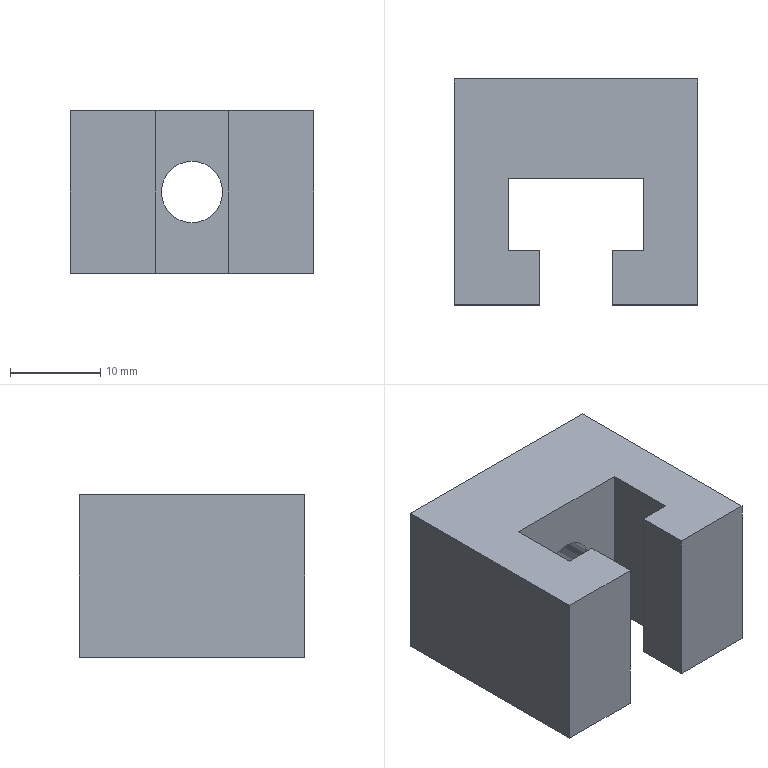Part | STEP file | iron shell displacement union seat | 1 solid | 16 faces | box 27 x 25 x 18 mm | volume 8727 mm3 | plane 14 | cylinder 2 | commonest cylinder face diameters 6.8 x2
STEP:
#1=CARTESIAN_POINT('',(0.,0.,0.));
#2=DIRECTION('',(0.,0.,1.));
#3=DIRECTION('',(1.,0.,0.));
#4=AXIS2_PLACEMENT_3D('',#1,#2,#3);
#5=CARTESIAN_POINT('',(-1856.966,-5970.89,12.4));
#6=VERTEX_POINT('',#5);
#7=CARTESIAN_POINT('',(-1856.966,-5959.89,12.4));
#8=VERTEX_POINT('',#7);
#9=CARTESIAN_POINT('',(-1856.966,-5959.89,12.4));
#10=DIRECTION('',(0.,1.,0.));
#11=VECTOR('',#10,1.);
#12=LINE('',#9,#11);
#13=CARTESIAN_POINT('',(-1856.966,-5959.89,9.));
#14=DIRECTION('',(0.,1.,0.));
#15=DIRECTION('',(0.,0.,1.));
#16=AXIS2_PLACEMENT_3D('',#13,#14,#15);
#17=CYLINDRICAL_SURFACE('',#16,3.4);
#18=CARTESIAN_POINT('',(6.283,0.));
#19=DIRECTION('',(0.,1.));
#20=VECTOR('',#19,1.);
#21=LINE('',#18,#20);
#22=(GEOMETRIC_REPRESENTATION_CONTEXT(2)PARAMETRIC_REPRESENTATION_CONTEXT()REPRESENTATION_CONTEXT('',''));
#23=DEFINITIONAL_REPRESENTATION('',(#21),#22);
#24=PCURVE('',#17,#23);
#25=CARTESIAN_POINT('',(-1856.966,-5959.89,9.));
#26=DIRECTION('',(0.,1.,0.));
#27=DIRECTION('',(0.,0.,1.));
#28=AXIS2_PLACEMENT_3D('',#25,#26,#27);
#29=CYLINDRICAL_SURFACE('',#28,3.4);
#30=CARTESIAN_POINT('',(0.,0.));
#31=DIRECTION('',(0.,1.));
#32=VECTOR('',#31,1.);
#33=LINE('',#30,#32);
#34=(GEOMETRIC_REPRESENTATION_CONTEXT(2)PARAMETRIC_REPRESENTATION_CONTEXT()REPRESENTATION_CONTEXT('',''));
#35=DEFINITIONAL_REPRESENTATION('',(#33),#34);
#36=PCURVE('',#29,#35);
#37=SURFACE_CURVE('',#12,(#24,#36),.PCURVE_S1.);
#38=EDGE_CURVE('',#6,#8,#37,.T.);
#39=ORIENTED_EDGE('',*,*,#38,.T.);
#40=CARTESIAN_POINT('',(-1856.966,-5959.89,5.6));
#41=VERTEX_POINT('',#40);
#42=CARTESIAN_POINT('',(-1856.966,-5959.89,9.));
#43=DIRECTION('',(0.,1.,0.));
#44=DIRECTION('',(0.,0.,1.));
#45=AXIS2_PLACEMENT_3D('',#42,#43,#44);
#46=CIRCLE('',#45,3.4);
#47=CARTESIAN_POINT('',(0.,0.));
#48=DIRECTION('',(1.,0.));
#49=VECTOR('',#48,1.);
#50=LINE('',#47,#49);
#51=(GEOMETRIC_REPRESENTATION_CONTEXT(2)PARAMETRIC_REPRESENTATION_CONTEXT()REPRESENTATION_CONTEXT('',''));
#52=DEFINITIONAL_REPRESENTATION('',(#50),#51);
#53=PCURVE('',#17,#52);
#54=CARTESIAN_POINT('',(-1870.466,-5959.89,18.));
#55=DIRECTION('',(0.,-1.,0.));
#56=DIRECTION('',(0.,0.,-1.));
#57=AXIS2_PLACEMENT_3D('',#54,#55,#56);
#58=PLANE('',#57);
#59=CARTESIAN_POINT('',(5.6,13.5));
#60=CARTESIAN_POINT('',(5.6,19.389));
#61=CARTESIAN_POINT('',(10.7,16.444));
#62=CARTESIAN_POINT('',(15.8,13.5));
#63=CARTESIAN_POINT('',(10.7,10.556));
#64=CARTESIAN_POINT('',(5.6,7.611));
#65=CARTESIAN_POINT('',(5.6,13.5));
#66=(BOUNDED_CURVE()B_SPLINE_CURVE(2,(#59,#60,#61,#62,#63,#64,#65),.UNSPECIFIED.,.T.,.F.)B_SPLINE_CURVE_WITH_KNOTS((1,2,2,2,2,1),(-2.094,0.,2.094,4.189,6.283,8.378),.UNSPECIFIED.)CURVE()GEOMETRIC_REPRESENTATION_ITEM()RATIONAL_B_SPLINE_CURVE((1.,0.5,1.,0.5,1.,0.5,1.))REPRESENTATION_ITEM(''));
#67=(GEOMETRIC_REPRESENTATION_CONTEXT(2)PARAMETRIC_REPRESENTATION_CONTEXT()REPRESENTATION_CONTEXT('',''));
#68=DEFINITIONAL_REPRESENTATION('',(#66),#67);
#69=PCURVE('',#58,#68);
#70=SURFACE_CURVE('',#46,(#53,#69),.PCURVE_S1.);
#71=EDGE_CURVE('',#41,#8,#70,.T.);
#72=ORIENTED_EDGE('',*,*,#71,.F.);
#73=CARTESIAN_POINT('',(-1856.966,-5970.89,5.6));
#74=VERTEX_POINT('',#73);
#75=CARTESIAN_POINT('',(-1856.966,-5959.89,5.6));
#76=DIRECTION('',(0.,1.,0.));
#77=VECTOR('',#76,1.);
#78=LINE('',#75,#77);
#79=CARTESIAN_POINT('',(3.142,0.));
#80=DIRECTION('',(0.,1.));
#81=VECTOR('',#80,1.);
#82=LINE('',#79,#81);
#83=(GEOMETRIC_REPRESENTATION_CONTEXT(2)PARAMETRIC_REPRESENTATION_CONTEXT()REPRESENTATION_CONTEXT('',''));
#84=DEFINITIONAL_REPRESENTATION('',(#82),#83);
#85=PCURVE('',#17,#84);
#86=CARTESIAN_POINT('',(3.142,0.));
#87=DIRECTION('',(0.,1.));
#88=VECTOR('',#87,1.);
#89=LINE('',#86,#88);
#90=(GEOMETRIC_REPRESENTATION_CONTEXT(2)PARAMETRIC_REPRESENTATION_CONTEXT()REPRESENTATION_CONTEXT('',''));
#91=DEFINITIONAL_REPRESENTATION('',(#89),#90);
#92=PCURVE('',#29,#91);
#93=SURFACE_CURVE('',#78,(#85,#92),.PCURVE_S1.);
#94=EDGE_CURVE('',#74,#41,#93,.T.);
#95=ORIENTED_EDGE('',*,*,#94,.F.);
#96=CARTESIAN_POINT('',(-1856.966,-5970.89,9.));
#97=DIRECTION('',(0.,1.,0.));
#98=DIRECTION('',(0.,0.,1.));
#99=AXIS2_PLACEMENT_3D('',#96,#97,#98);
#100=CIRCLE('',#99,3.4);
#101=CARTESIAN_POINT('',(0.,-11.));
#102=DIRECTION('',(1.,0.));
#103=VECTOR('',#102,1.);
#104=LINE('',#101,#103);
#105=(GEOMETRIC_REPRESENTATION_CONTEXT(2)PARAMETRIC_REPRESENTATION_CONTEXT()REPRESENTATION_CONTEXT('',''));
#106=DEFINITIONAL_REPRESENTATION('',(#104),#105);
#107=PCURVE('',#17,#106);
#108=CARTESIAN_POINT('',(-1849.466,-5970.89,18.));
#109=DIRECTION('',(0.,1.,0.));
#110=DIRECTION('',(0.,0.,1.));
#111=AXIS2_PLACEMENT_3D('',#108,#109,#110);
#112=PLANE('',#111);
#113=CARTESIAN_POINT('',(-9.,-7.5));
#114=DIRECTION('',(1.,0.));
#115=AXIS2_PLACEMENT_2D('',#113,#114);
#116=CIRCLE('',#115,3.4);
#117=(GEOMETRIC_REPRESENTATION_CONTEXT(2)PARAMETRIC_REPRESENTATION_CONTEXT()REPRESENTATION_CONTEXT('',''));
#118=DEFINITIONAL_REPRESENTATION('',(#116),#117);
#119=PCURVE('',#112,#118);
#120=SURFACE_CURVE('',#100,(#107,#119),.PCURVE_S1.);
#121=EDGE_CURVE('',#74,#6,#120,.T.);
#122=ORIENTED_EDGE('',*,*,#121,.T.);
#123=EDGE_LOOP('',(#39,#72,#95,#122));
#124=FACE_BOUND('',#123,.F.);
#125=ADVANCED_FACE('',(#124),#17,.F.);
#126=CARTESIAN_POINT('',(-1856.966,-5959.89,9.));
#127=DIRECTION('',(0.,1.,0.));
#128=DIRECTION('',(0.,0.,1.));
#129=AXIS2_PLACEMENT_3D('',#126,#127,#128);
#130=CIRCLE('',#129,3.4);
#131=CARTESIAN_POINT('',(5.6,13.5));
#132=CARTESIAN_POINT('',(5.6,19.389));
#133=CARTESIAN_POINT('',(10.7,16.444));
#134=CARTESIAN_POINT('',(15.8,13.5));
#135=CARTESIAN_POINT('',(10.7,10.556));
#136=CARTESIAN_POINT('',(5.6,7.611));
#137=CARTESIAN_POINT('',(5.6,13.5));
#138=(BOUNDED_CURVE()B_SPLINE_CURVE(2,(#131,#132,#133,#134,#135,#136,#137),.UNSPECIFIED.,.T.,.F.)B_SPLINE_CURVE_WITH_KNOTS((1,2,2,2,2,1),(-2.094,0.,2.094,4.189,6.283,8.378),.UNSPECIFIED.)CURVE()GEOMETRIC_REPRESENTATION_ITEM()RATIONAL_B_SPLINE_CURVE((1.,0.5,1.,0.5,1.,0.5,1.))REPRESENTATION_ITEM(''));
#139=(GEOMETRIC_REPRESENTATION_CONTEXT(2)PARAMETRIC_REPRESENTATION_CONTEXT()REPRESENTATION_CONTEXT('',''));
#140=DEFINITIONAL_REPRESENTATION('',(#138),#139);
#141=PCURVE('',#58,#140);
#142=CARTESIAN_POINT('',(0.,0.));
#143=DIRECTION('',(1.,0.));
#144=VECTOR('',#143,1.);
#145=LINE('',#142,#144);
#146=(GEOMETRIC_REPRESENTATION_CONTEXT(2)PARAMETRIC_REPRESENTATION_CONTEXT()REPRESENTATION_CONTEXT('',''));
#147=DEFINITIONAL_REPRESENTATION('',(#145),#146);
#148=PCURVE('',#29,#147);
#149=SURFACE_CURVE('',#130,(#141,#148),.PCURVE_S1.);
#150=EDGE_CURVE('',#8,#41,#149,.T.);
#151=ORIENTED_EDGE('',*,*,#150,.F.);
#152=ORIENTED_EDGE('',*,*,#71,.F.);
#153=EDGE_LOOP('',(#151,#152));
#154=FACE_BOUND('',#153,.T.);
#155=CARTESIAN_POINT('',(-1843.466,-5959.89,0.));
#156=VERTEX_POINT('',#155);
#157=CARTESIAN_POINT('',(-1870.466,-5959.89,0.));
#158=VERTEX_POINT('',#157);
#159=CARTESIAN_POINT('',(-1870.466,-5959.89,0.));
#160=DIRECTION('',(-1.,0.,0.));
#161=VECTOR('',#160,1.);
#162=LINE('',#159,#161);
#163=CARTESIAN_POINT('',(18.,0.));
#164=DIRECTION('',(0.,-1.));
#165=VECTOR('',#164,1.);
#166=LINE('',#163,#165);
#167=(GEOMETRIC_REPRESENTATION_CONTEXT(2)PARAMETRIC_REPRESENTATION_CONTEXT()REPRESENTATION_CONTEXT('',''));
#168=DEFINITIONAL_REPRESENTATION('',(#166),#167);
#169=PCURVE('',#58,#168);
#170=CARTESIAN_POINT('',(-1843.466,-5959.89,0.));
#171=DIRECTION('',(0.,0.,-1.));
#172=DIRECTION('',(-1.,0.,0.));
#173=AXIS2_PLACEMENT_3D('',#170,#171,#172);
#174=PLANE('',#173);
#175=CARTESIAN_POINT('',(27.,0.));
#176=DIRECTION('',(1.,0.));
#177=VECTOR('',#176,1.);
#178=LINE('',#175,#177);
#179=(GEOMETRIC_REPRESENTATION_CONTEXT(2)PARAMETRIC_REPRESENTATION_CONTEXT()REPRESENTATION_CONTEXT('',''));
#180=DEFINITIONAL_REPRESENTATION('',(#178),#179);
#181=PCURVE('',#174,#180);
#182=SURFACE_CURVE('',#162,(#169,#181),.PCURVE_S1.);
#183=EDGE_CURVE('',#156,#158,#182,.T.);
#184=ORIENTED_EDGE('',*,*,#183,.T.);
#185=CARTESIAN_POINT('',(-1870.466,-5959.89,18.));
#186=VERTEX_POINT('',#185);
#187=CARTESIAN_POINT('',(-1870.466,-5959.89,18.));
#188=DIRECTION('',(0.,0.,-1.));
#189=VECTOR('',#188,1.);
#190=LINE('',#187,#189);
#191=CARTESIAN_POINT('',(0.,0.));
#192=DIRECTION('',(1.,0.));
#193=VECTOR('',#192,1.);
#194=LINE('',#191,#193);
#195=(GEOMETRIC_REPRESENTATION_CONTEXT(2)PARAMETRIC_REPRESENTATION_CONTEXT()REPRESENTATION_CONTEXT('',''));
#196=DEFINITIONAL_REPRESENTATION('',(#194),#195);
#197=PCURVE('',#58,#196);
#198=CARTESIAN_POINT('',(-1870.466,-5959.89,18.));
#199=DIRECTION('',(1.,0.,0.));
#200=DIRECTION('',(0.,0.,-1.));
#201=AXIS2_PLACEMENT_3D('',#198,#199,#200);
#202=PLANE('',#201);
#203=CARTESIAN_POINT('',(0.,0.));
#204=DIRECTION('',(1.,0.));
#205=VECTOR('',#204,1.);
#206=LINE('',#203,#205);
#207=(GEOMETRIC_REPRESENTATION_CONTEXT(2)PARAMETRIC_REPRESENTATION_CONTEXT()REPRESENTATION_CONTEXT('',''));
#208=DEFINITIONAL_REPRESENTATION('',(#206),#207);
#209=PCURVE('',#202,#208);
#210=SURFACE_CURVE('',#190,(#197,#209),.PCURVE_S1.);
#211=EDGE_CURVE('',#186,#158,#210,.T.);
#212=ORIENTED_EDGE('',*,*,#211,.F.);
#213=CARTESIAN_POINT('',(-1843.466,-5959.89,18.));
#214=VERTEX_POINT('',#213);
#215=CARTESIAN_POINT('',(-1870.466,-5959.89,18.));
#216=DIRECTION('',(-1.,0.,0.));
#217=VECTOR('',#216,1.);
#218=LINE('',#215,#217);
#219=CARTESIAN_POINT('',(0.,0.));
#220=DIRECTION('',(0.,-1.));
#221=VECTOR('',#220,1.);
#222=LINE('',#219,#221);
#223=(GEOMETRIC_REPRESENTATION_CONTEXT(2)PARAMETRIC_REPRESENTATION_CONTEXT()REPRESENTATION_CONTEXT('',''));
#224=DEFINITIONAL_REPRESENTATION('',(#222),#223);
#225=PCURVE('',#58,#224);
#226=CARTESIAN_POINT('',(-1843.466,-5959.89,18.));
#227=DIRECTION('',(0.,0.,-1.));
#228=DIRECTION('',(-1.,0.,0.));
#229=AXIS2_PLACEMENT_3D('',#226,#227,#228);
#230=PLANE('',#229);
#231=CARTESIAN_POINT('',(27.,0.));
#232=DIRECTION('',(1.,0.));
#233=VECTOR('',#232,1.);
#234=LINE('',#231,#233);
#235=(GEOMETRIC_REPRESENTATION_CONTEXT(2)PARAMETRIC_REPRESENTATION_CONTEXT()REPRESENTATION_CONTEXT('',''));
#236=DEFINITIONAL_REPRESENTATION('',(#234),#235);
#237=PCURVE('',#230,#236);
#238=SURFACE_CURVE('',#218,(#225,#237),.PCURVE_S1.);
#239=EDGE_CURVE('',#214,#186,#238,.T.);
#240=ORIENTED_EDGE('',*,*,#239,.F.);
#241=CARTESIAN_POINT('',(-1843.466,-5959.89,18.));
#242=DIRECTION('',(0.,0.,-1.));
#243=VECTOR('',#242,1.);
#244=LINE('',#241,#243);
#245=CARTESIAN_POINT('',(0.,27.));
#246=DIRECTION('',(1.,0.));
#247=VECTOR('',#246,1.);
#248=LINE('',#245,#247);
#249=(GEOMETRIC_REPRESENTATION_CONTEXT(2)PARAMETRIC_REPRESENTATION_CONTEXT()REPRESENTATION_CONTEXT('',''));
#250=DEFINITIONAL_REPRESENTATION('',(#248),#249);
#251=PCURVE('',#58,#250);
#252=CARTESIAN_POINT('',(-1843.466,-5959.89,18.));
#253=DIRECTION('',(-1.,0.,0.));
#254=DIRECTION('',(0.,0.,1.));
#255=AXIS2_PLACEMENT_3D('',#252,#253,#254);
#256=PLANE('',#255);
#257=CARTESIAN_POINT('',(0.,0.));
#258=DIRECTION('',(-1.,0.));
#259=VECTOR('',#258,1.);
#260=LINE('',#257,#259);
#261=(GEOMETRIC_REPRESENTATION_CONTEXT(2)PARAMETRIC_REPRESENTATION_CONTEXT()REPRESENTATION_CONTEXT('',''));
#262=DEFINITIONAL_REPRESENTATION('',(#260),#261);
#263=PCURVE('',#256,#262);
#264=SURFACE_CURVE('',#244,(#251,#263),.PCURVE_S1.);
#265=EDGE_CURVE('',#214,#156,#264,.T.);
#266=ORIENTED_EDGE('',*,*,#265,.T.);
#267=EDGE_LOOP('',(#184,#212,#240,#266));
#268=FACE_BOUND('',#267,.T.);
#269=ADVANCED_FACE('',(#154,#268),#58,.F.);
#270=CARTESIAN_POINT('',(-1870.466,-5984.89,0.));
#271=VERTEX_POINT('',#270);
#272=CARTESIAN_POINT('',(-1870.466,-5959.89,0.));
#273=DIRECTION('',(0.,-1.,0.));
#274=VECTOR('',#273,1.);
#275=LINE('',#272,#274);
#276=CARTESIAN_POINT('',(18.,0.));
#277=DIRECTION('',(0.,-1.));
#278=VECTOR('',#277,1.);
#279=LINE('',#276,#278);
#280=(GEOMETRIC_REPRESENTATION_CONTEXT(2)PARAMETRIC_REPRESENTATION_CONTEXT()REPRESENTATION_CONTEXT('',''));
#281=DEFINITIONAL_REPRESENTATION('',(#279),#280);
#282=PCURVE('',#202,#281);
#283=CARTESIAN_POINT('',(27.,0.));
#284=DIRECTION('',(0.,-1.));
#285=VECTOR('',#284,1.);
#286=LINE('',#283,#285);
#287=(GEOMETRIC_REPRESENTATION_CONTEXT(2)PARAMETRIC_REPRESENTATION_CONTEXT()REPRESENTATION_CONTEXT('',''));
#288=DEFINITIONAL_REPRESENTATION('',(#286),#287);
#289=PCURVE('',#174,#288);
#290=SURFACE_CURVE('',#275,(#282,#289),.PCURVE_S1.);
#291=EDGE_CURVE('',#158,#271,#290,.T.);
#292=ORIENTED_EDGE('',*,*,#291,.T.);
#293=CARTESIAN_POINT('',(-1870.466,-5984.89,18.));
#294=VERTEX_POINT('',#293);
#295=CARTESIAN_POINT('',(-1870.466,-5984.89,18.));
#296=DIRECTION('',(0.,0.,-1.));
#297=VECTOR('',#296,1.);
#298=LINE('',#295,#297);
#299=CARTESIAN_POINT('',(0.,-25.));
#300=DIRECTION('',(1.,0.));
#301=VECTOR('',#300,1.);
#302=LINE('',#299,#301);
#303=(GEOMETRIC_REPRESENTATION_CONTEXT(2)PARAMETRIC_REPRESENTATION_CONTEXT()REPRESENTATION_CONTEXT('',''));
#304=DEFINITIONAL_REPRESENTATION('',(#302),#303);
#305=PCURVE('',#202,#304);
#306=CARTESIAN_POINT('',(-1860.966,-5984.89,18.));
#307=DIRECTION('',(0.,1.,0.));
#308=DIRECTION('',(0.,0.,1.));
#309=AXIS2_PLACEMENT_3D('',#306,#307,#308);
#310=PLANE('',#309);
#311=CARTESIAN_POINT('',(0.,-9.5));
#312=DIRECTION('',(-1.,0.));
#313=VECTOR('',#312,1.);
#314=LINE('',#311,#313);
#315=(GEOMETRIC_REPRESENTATION_CONTEXT(2)PARAMETRIC_REPRESENTATION_CONTEXT()REPRESENTATION_CONTEXT('',''));
#316=DEFINITIONAL_REPRESENTATION('',(#314),#315);
#317=PCURVE('',#310,#316);
#318=SURFACE_CURVE('',#298,(#305,#317),.PCURVE_S1.);
#319=EDGE_CURVE('',#294,#271,#318,.T.);
#320=ORIENTED_EDGE('',*,*,#319,.F.);
#321=CARTESIAN_POINT('',(-1870.466,-5959.89,18.));
#322=DIRECTION('',(0.,-1.,0.));
#323=VECTOR('',#322,1.);
#324=LINE('',#321,#323);
#325=CARTESIAN_POINT('',(0.,0.));
#326=DIRECTION('',(0.,-1.));
#327=VECTOR('',#326,1.);
#328=LINE('',#325,#327);
#329=(GEOMETRIC_REPRESENTATION_CONTEXT(2)PARAMETRIC_REPRESENTATION_CONTEXT()REPRESENTATION_CONTEXT('',''));
#330=DEFINITIONAL_REPRESENTATION('',(#328),#329);
#331=PCURVE('',#202,#330);
#332=CARTESIAN_POINT('',(27.,0.));
#333=DIRECTION('',(0.,-1.));
#334=VECTOR('',#333,1.);
#335=LINE('',#332,#334);
#336=(GEOMETRIC_REPRESENTATION_CONTEXT(2)PARAMETRIC_REPRESENTATION_CONTEXT()REPRESENTATION_CONTEXT('',''));
#337=DEFINITIONAL_REPRESENTATION('',(#335),#336);
#338=PCURVE('',#230,#337);
#339=SURFACE_CURVE('',#324,(#331,#338),.PCURVE_S1.);
#340=EDGE_CURVE('',#186,#294,#339,.T.);
#341=ORIENTED_EDGE('',*,*,#340,.F.);
#342=ORIENTED_EDGE('',*,*,#211,.T.);
#343=EDGE_LOOP('',(#292,#320,#341,#342));
#344=FACE_BOUND('',#343,.T.);
#345=ADVANCED_FACE('',(#344),#202,.F.);
#346=CARTESIAN_POINT('',(-1860.966,-5984.89,0.));
#347=VERTEX_POINT('',#346);
#348=CARTESIAN_POINT('',(-1860.966,-5984.89,0.));
#349=DIRECTION('',(1.,0.,0.));
#350=VECTOR('',#349,1.);
#351=LINE('',#348,#350);
#352=CARTESIAN_POINT('',(-18.,0.));
#353=DIRECTION('',(0.,1.));
#354=VECTOR('',#353,1.);
#355=LINE('',#352,#354);
#356=(GEOMETRIC_REPRESENTATION_CONTEXT(2)PARAMETRIC_REPRESENTATION_CONTEXT()REPRESENTATION_CONTEXT('',''));
#357=DEFINITIONAL_REPRESENTATION('',(#355),#356);
#358=PCURVE('',#310,#357);
#359=CARTESIAN_POINT('',(17.5,-25.));
#360=DIRECTION('',(-1.,0.));
#361=VECTOR('',#360,1.);
#362=LINE('',#359,#361);
#363=(GEOMETRIC_REPRESENTATION_CONTEXT(2)PARAMETRIC_REPRESENTATION_CONTEXT()REPRESENTATION_CONTEXT('',''));
#364=DEFINITIONAL_REPRESENTATION('',(#362),#363);
#365=PCURVE('',#174,#364);
#366=SURFACE_CURVE('',#351,(#358,#365),.PCURVE_S1.);
#367=EDGE_CURVE('',#271,#347,#366,.T.);
#368=ORIENTED_EDGE('',*,*,#367,.T.);
#369=CARTESIAN_POINT('',(-1860.966,-5984.89,18.));
#370=VERTEX_POINT('',#369);
#371=CARTESIAN_POINT('',(-1860.966,-5984.89,18.));
#372=DIRECTION('',(0.,0.,-1.));
#373=VECTOR('',#372,1.);
#374=LINE('',#371,#373);
#375=CARTESIAN_POINT('',(0.,0.));
#376=DIRECTION('',(-1.,0.));
#377=VECTOR('',#376,1.);
#378=LINE('',#375,#377);
#379=(GEOMETRIC_REPRESENTATION_CONTEXT(2)PARAMETRIC_REPRESENTATION_CONTEXT()REPRESENTATION_CONTEXT('',''));
#380=DEFINITIONAL_REPRESENTATION('',(#378),#379);
#381=PCURVE('',#310,#380);
#382=CARTESIAN_POINT('',(-1860.966,-5978.89,18.));
#383=DIRECTION('',(-1.,0.,0.));
#384=DIRECTION('',(0.,0.,1.));
#385=AXIS2_PLACEMENT_3D('',#382,#383,#384);
#386=PLANE('',#385);
#387=CARTESIAN_POINT('',(0.,-6.));
#388=DIRECTION('',(-1.,0.));
#389=VECTOR('',#388,1.);
#390=LINE('',#387,#389);
#391=(GEOMETRIC_REPRESENTATION_CONTEXT(2)PARAMETRIC_REPRESENTATION_CONTEXT()REPRESENTATION_CONTEXT('',''));
#392=DEFINITIONAL_REPRESENTATION('',(#390),#391);
#393=PCURVE('',#386,#392);
#394=SURFACE_CURVE('',#374,(#381,#393),.PCURVE_S1.);
#395=EDGE_CURVE('',#370,#347,#394,.T.);
#396=ORIENTED_EDGE('',*,*,#395,.F.);
#397=CARTESIAN_POINT('',(-1860.966,-5984.89,18.));
#398=DIRECTION('',(1.,0.,0.));
#399=VECTOR('',#398,1.);
#400=LINE('',#397,#399);
#401=CARTESIAN_POINT('',(0.,0.));
#402=DIRECTION('',(0.,1.));
#403=VECTOR('',#402,1.);
#404=LINE('',#401,#403);
#405=(GEOMETRIC_REPRESENTATION_CONTEXT(2)PARAMETRIC_REPRESENTATION_CONTEXT()REPRESENTATION_CONTEXT('',''));
#406=DEFINITIONAL_REPRESENTATION('',(#404),#405);
#407=PCURVE('',#310,#406);
#408=CARTESIAN_POINT('',(17.5,-25.));
#409=DIRECTION('',(-1.,0.));
#410=VECTOR('',#409,1.);
#411=LINE('',#408,#410);
#412=(GEOMETRIC_REPRESENTATION_CONTEXT(2)PARAMETRIC_REPRESENTATION_CONTEXT()REPRESENTATION_CONTEXT('',''));
#413=DEFINITIONAL_REPRESENTATION('',(#411),#412);
#414=PCURVE('',#230,#413);
#415=SURFACE_CURVE('',#400,(#407,#414),.PCURVE_S1.);
#416=EDGE_CURVE('',#294,#370,#415,.T.);
#417=ORIENTED_EDGE('',*,*,#416,.F.);
#418=ORIENTED_EDGE('',*,*,#319,.T.);
#419=EDGE_LOOP('',(#368,#396,#417,#418));
#420=FACE_BOUND('',#419,.T.);
#421=ADVANCED_FACE('',(#420),#310,.F.);
#422=CARTESIAN_POINT('',(-1860.966,-5978.89,0.));
#423=VERTEX_POINT('',#422);
#424=CARTESIAN_POINT('',(-1860.966,-5978.89,0.));
#425=DIRECTION('',(0.,1.,0.));
#426=VECTOR('',#425,1.);
#427=LINE('',#424,#426);
#428=CARTESIAN_POINT('',(-18.,0.));
#429=DIRECTION('',(0.,1.));
#430=VECTOR('',#429,1.);
#431=LINE('',#428,#430);
#432=(GEOMETRIC_REPRESENTATION_CONTEXT(2)PARAMETRIC_REPRESENTATION_CONTEXT()REPRESENTATION_CONTEXT('',''));
#433=DEFINITIONAL_REPRESENTATION('',(#431),#432);
#434=PCURVE('',#386,#433);
#435=CARTESIAN_POINT('',(17.5,-19.));
#436=DIRECTION('',(0.,1.));
#437=VECTOR('',#436,1.);
#438=LINE('',#435,#437);
#439=(GEOMETRIC_REPRESENTATION_CONTEXT(2)PARAMETRIC_REPRESENTATION_CONTEXT()REPRESENTATION_CONTEXT('',''));
#440=DEFINITIONAL_REPRESENTATION('',(#438),#439);
#441=PCURVE('',#174,#440);
#442=SURFACE_CURVE('',#427,(#434,#441),.PCURVE_S1.);
#443=EDGE_CURVE('',#347,#423,#442,.T.);
#444=ORIENTED_EDGE('',*,*,#443,.T.);
#445=CARTESIAN_POINT('',(-1860.966,-5978.89,18.));
#446=VERTEX_POINT('',#445);
#447=CARTESIAN_POINT('',(-1860.966,-5978.89,18.));
#448=DIRECTION('',(0.,0.,-1.));
#449=VECTOR('',#448,1.);
#450=LINE('',#447,#449);
#451=CARTESIAN_POINT('',(0.,0.));
#452=DIRECTION('',(-1.,0.));
#453=VECTOR('',#452,1.);
#454=LINE('',#451,#453);
#455=(GEOMETRIC_REPRESENTATION_CONTEXT(2)PARAMETRIC_REPRESENTATION_CONTEXT()REPRESENTATION_CONTEXT('',''));
#456=DEFINITIONAL_REPRESENTATION('',(#454),#455);
#457=PCURVE('',#386,#456);
#458=CARTESIAN_POINT('',(-1864.466,-5978.89,18.));
#459=DIRECTION('',(0.,-1.,0.));
#460=DIRECTION('',(0.,0.,-1.));
#461=AXIS2_PLACEMENT_3D('',#458,#459,#460);
#462=PLANE('',#461);
#463=CARTESIAN_POINT('',(0.,3.5));
#464=DIRECTION('',(1.,0.));
#465=VECTOR('',#464,1.);
#466=LINE('',#463,#465);
#467=(GEOMETRIC_REPRESENTATION_CONTEXT(2)PARAMETRIC_REPRESENTATION_CONTEXT()REPRESENTATION_CONTEXT('',''));
#468=DEFINITIONAL_REPRESENTATION('',(#466),#467);
#469=PCURVE('',#462,#468);
#470=SURFACE_CURVE('',#450,(#457,#469),.PCURVE_S1.);
#471=EDGE_CURVE('',#446,#423,#470,.T.);
#472=ORIENTED_EDGE('',*,*,#471,.F.);
#473=CARTESIAN_POINT('',(-1860.966,-5978.89,18.));
#474=DIRECTION('',(0.,1.,0.));
#475=VECTOR('',#474,1.);
#476=LINE('',#473,#475);
#477=CARTESIAN_POINT('',(0.,0.));
#478=DIRECTION('',(0.,1.));
#479=VECTOR('',#478,1.);
#480=LINE('',#477,#479);
#481=(GEOMETRIC_REPRESENTATION_CONTEXT(2)PARAMETRIC_REPRESENTATION_CONTEXT()REPRESENTATION_CONTEXT('',''));
#482=DEFINITIONAL_REPRESENTATION('',(#480),#481);
#483=PCURVE('',#386,#482);
#484=CARTESIAN_POINT('',(17.5,-19.));
#485=DIRECTION('',(0.,1.));
#486=VECTOR('',#485,1.);
#487=LINE('',#484,#486);
#488=(GEOMETRIC_REPRESENTATION_CONTEXT(2)PARAMETRIC_REPRESENTATION_CONTEXT()REPRESENTATION_CONTEXT('',''));
#489=DEFINITIONAL_REPRESENTATION('',(#487),#488);
#490=PCURVE('',#230,#489);
#491=SURFACE_CURVE('',#476,(#483,#490),.PCURVE_S1.);
#492=EDGE_CURVE('',#370,#446,#491,.T.);
#493=ORIENTED_EDGE('',*,*,#492,.F.);
#494=ORIENTED_EDGE('',*,*,#395,.T.);
#495=EDGE_LOOP('',(#444,#472,#493,#494));
#496=FACE_BOUND('',#495,.T.);
#497=ADVANCED_FACE('',(#496),#386,.F.);
#498=CARTESIAN_POINT('',(-1864.466,-5978.89,0.));
#499=VERTEX_POINT('',#498);
#500=CARTESIAN_POINT('',(-1864.466,-5978.89,0.));
#501=DIRECTION('',(-1.,0.,0.));
#502=VECTOR('',#501,1.);
#503=LINE('',#500,#502);
#504=CARTESIAN_POINT('',(18.,0.));
#505=DIRECTION('',(0.,-1.));
#506=VECTOR('',#505,1.);
#507=LINE('',#504,#506);
#508=(GEOMETRIC_REPRESENTATION_CONTEXT(2)PARAMETRIC_REPRESENTATION_CONTEXT()REPRESENTATION_CONTEXT('',''));
#509=DEFINITIONAL_REPRESENTATION('',(#507),#508);
#510=PCURVE('',#462,#509);
#511=CARTESIAN_POINT('',(21.,-19.));
#512=DIRECTION('',(1.,0.));
#513=VECTOR('',#512,1.);
#514=LINE('',#511,#513);
#515=(GEOMETRIC_REPRESENTATION_CONTEXT(2)PARAMETRIC_REPRESENTATION_CONTEXT()REPRESENTATION_CONTEXT('',''));
#516=DEFINITIONAL_REPRESENTATION('',(#514),#515);
#517=PCURVE('',#174,#516);
#518=SURFACE_CURVE('',#503,(#510,#517),.PCURVE_S1.);
#519=EDGE_CURVE('',#423,#499,#518,.T.);
#520=ORIENTED_EDGE('',*,*,#519,.T.);
#521=CARTESIAN_POINT('',(-1864.466,-5978.89,18.));
#522=VERTEX_POINT('',#521);
#523=CARTESIAN_POINT('',(-1864.466,-5978.89,18.));
#524=DIRECTION('',(0.,0.,-1.));
#525=VECTOR('',#524,1.);
#526=LINE('',#523,#525);
#527=CARTESIAN_POINT('',(0.,0.));
#528=DIRECTION('',(1.,0.));
#529=VECTOR('',#528,1.);
#530=LINE('',#527,#529);
#531=(GEOMETRIC_REPRESENTATION_CONTEXT(2)PARAMETRIC_REPRESENTATION_CONTEXT()REPRESENTATION_CONTEXT('',''));
#532=DEFINITIONAL_REPRESENTATION('',(#530),#531);
#533=PCURVE('',#462,#532);
#534=CARTESIAN_POINT('',(-1864.466,-5970.89,18.));
#535=DIRECTION('',(-1.,0.,0.));
#536=DIRECTION('',(0.,0.,1.));
#537=AXIS2_PLACEMENT_3D('',#534,#535,#536);
#538=PLANE('',#537);
#539=CARTESIAN_POINT('',(0.,-8.));
#540=DIRECTION('',(-1.,0.));
#541=VECTOR('',#540,1.);
#542=LINE('',#539,#541);
#543=(GEOMETRIC_REPRESENTATION_CONTEXT(2)PARAMETRIC_REPRESENTATION_CONTEXT()REPRESENTATION_CONTEXT('',''));
#544=DEFINITIONAL_REPRESENTATION('',(#542),#543);
#545=PCURVE('',#538,#544);
#546=SURFACE_CURVE('',#526,(#533,#545),.PCURVE_S1.);
#547=EDGE_CURVE('',#522,#499,#546,.T.);
#548=ORIENTED_EDGE('',*,*,#547,.F.);
#549=CARTESIAN_POINT('',(-1864.466,-5978.89,18.));
#550=DIRECTION('',(-1.,0.,0.));
#551=VECTOR('',#550,1.);
#552=LINE('',#549,#551);
#553=CARTESIAN_POINT('',(0.,0.));
#554=DIRECTION('',(0.,-1.));
#555=VECTOR('',#554,1.);
#556=LINE('',#553,#555);
#557=(GEOMETRIC_REPRESENTATION_CONTEXT(2)PARAMETRIC_REPRESENTATION_CONTEXT()REPRESENTATION_CONTEXT('',''));
#558=DEFINITIONAL_REPRESENTATION('',(#556),#557);
#559=PCURVE('',#462,#558);
#560=CARTESIAN_POINT('',(21.,-19.));
#561=DIRECTION('',(1.,0.));
#562=VECTOR('',#561,1.);
#563=LINE('',#560,#562);
#564=(GEOMETRIC_REPRESENTATION_CONTEXT(2)PARAMETRIC_REPRESENTATION_CONTEXT()REPRESENTATION_CONTEXT('',''));
#565=DEFINITIONAL_REPRESENTATION('',(#563),#564);
#566=PCURVE('',#230,#565);
#567=SURFACE_CURVE('',#552,(#559,#566),.PCURVE_S1.);
#568=EDGE_CURVE('',#446,#522,#567,.T.);
#569=ORIENTED_EDGE('',*,*,#568,.F.);
#570=ORIENTED_EDGE('',*,*,#471,.T.);
#571=EDGE_LOOP('',(#520,#548,#569,#570));
#572=FACE_BOUND('',#571,.T.);
#573=ADVANCED_FACE('',(#572),#462,.F.);
#574=CARTESIAN_POINT('',(-1864.466,-5970.89,0.));
#575=VERTEX_POINT('',#574);
#576=CARTESIAN_POINT('',(-1864.466,-5970.89,0.));
#577=DIRECTION('',(0.,1.,0.));
#578=VECTOR('',#577,1.);
#579=LINE('',#576,#578);
#580=CARTESIAN_POINT('',(-18.,0.));
#581=DIRECTION('',(0.,1.));
#582=VECTOR('',#581,1.);
#583=LINE('',#580,#582);
#584=(GEOMETRIC_REPRESENTATION_CONTEXT(2)PARAMETRIC_REPRESENTATION_CONTEXT()REPRESENTATION_CONTEXT('',''));
#585=DEFINITIONAL_REPRESENTATION('',(#583),#584);
#586=PCURVE('',#538,#585);
#587=CARTESIAN_POINT('',(21.,-11.));
#588=DIRECTION('',(0.,1.));
#589=VECTOR('',#588,1.);
#590=LINE('',#587,#589);
#591=(GEOMETRIC_REPRESENTATION_CONTEXT(2)PARAMETRIC_REPRESENTATION_CONTEXT()REPRESENTATION_CONTEXT('',''));
#592=DEFINITIONAL_REPRESENTATION('',(#590),#591);
#593=PCURVE('',#174,#592);
#594=SURFACE_CURVE('',#579,(#586,#593),.PCURVE_S1.);
#595=EDGE_CURVE('',#499,#575,#594,.T.);
#596=ORIENTED_EDGE('',*,*,#595,.T.);
#597=CARTESIAN_POINT('',(-1864.466,-5970.89,18.));
#598=VERTEX_POINT('',#597);
#599=CARTESIAN_POINT('',(-1864.466,-5970.89,18.));
#600=DIRECTION('',(0.,0.,-1.));
#601=VECTOR('',#600,1.);
#602=LINE('',#599,#601);
#603=CARTESIAN_POINT('',(0.,0.));
#604=DIRECTION('',(-1.,0.));
#605=VECTOR('',#604,1.);
#606=LINE('',#603,#605);
#607=(GEOMETRIC_REPRESENTATION_CONTEXT(2)PARAMETRIC_REPRESENTATION_CONTEXT()REPRESENTATION_CONTEXT('',''));
#608=DEFINITIONAL_REPRESENTATION('',(#606),#607);
#609=PCURVE('',#538,#608);
#610=CARTESIAN_POINT('',(0.,-15.));
#611=DIRECTION('',(-1.,0.));
#612=VECTOR('',#611,1.);
#613=LINE('',#610,#612);
#614=(GEOMETRIC_REPRESENTATION_CONTEXT(2)PARAMETRIC_REPRESENTATION_CONTEXT()REPRESENTATION_CONTEXT('',''));
#615=DEFINITIONAL_REPRESENTATION('',(#613),#614);
#616=PCURVE('',#112,#615);
#617=SURFACE_CURVE('',#602,(#609,#616),.PCURVE_S1.);
#618=EDGE_CURVE('',#598,#575,#617,.T.);
#619=ORIENTED_EDGE('',*,*,#618,.F.);
#620=CARTESIAN_POINT('',(-1864.466,-5970.89,18.));
#621=DIRECTION('',(0.,1.,0.));
#622=VECTOR('',#621,1.);
#623=LINE('',#620,#622);
#624=CARTESIAN_POINT('',(0.,0.));
#625=DIRECTION('',(0.,1.));
#626=VECTOR('',#625,1.);
#627=LINE('',#624,#626);
#628=(GEOMETRIC_REPRESENTATION_CONTEXT(2)PARAMETRIC_REPRESENTATION_CONTEXT()REPRESENTATION_CONTEXT('',''));
#629=DEFINITIONAL_REPRESENTATION('',(#627),#628);
#630=PCURVE('',#538,#629);
#631=CARTESIAN_POINT('',(21.,-11.));
#632=DIRECTION('',(0.,1.));
#633=VECTOR('',#632,1.);
#634=LINE('',#631,#633);
#635=(GEOMETRIC_REPRESENTATION_CONTEXT(2)PARAMETRIC_REPRESENTATION_CONTEXT()REPRESENTATION_CONTEXT('',''));
#636=DEFINITIONAL_REPRESENTATION('',(#634),#635);
#637=PCURVE('',#230,#636);
#638=SURFACE_CURVE('',#623,(#630,#637),.PCURVE_S1.);
#639=EDGE_CURVE('',#522,#598,#638,.T.);
#640=ORIENTED_EDGE('',*,*,#639,.F.);
#641=ORIENTED_EDGE('',*,*,#547,.T.);
#642=EDGE_LOOP('',(#596,#619,#640,#641));
#643=FACE_BOUND('',#642,.T.);
#644=ADVANCED_FACE('',(#643),#538,.F.);
#645=CARTESIAN_POINT('',(-1856.966,-5970.89,9.));
#646=DIRECTION('',(0.,1.,0.));
#647=DIRECTION('',(0.,0.,1.));
#648=AXIS2_PLACEMENT_3D('',#645,#646,#647);
#649=CIRCLE('',#648,3.4);
#650=CARTESIAN_POINT('',(-9.,-7.5));
#651=DIRECTION('',(1.,0.));
#652=AXIS2_PLACEMENT_2D('',#650,#651);
#653=CIRCLE('',#652,3.4);
#654=(GEOMETRIC_REPRESENTATION_CONTEXT(2)PARAMETRIC_REPRESENTATION_CONTEXT()REPRESENTATION_CONTEXT('',''));
#655=DEFINITIONAL_REPRESENTATION('',(#653),#654);
#656=PCURVE('',#112,#655);
#657=CARTESIAN_POINT('',(0.,-11.));
#658=DIRECTION('',(1.,0.));
#659=VECTOR('',#658,1.);
#660=LINE('',#657,#659);
#661=(GEOMETRIC_REPRESENTATION_CONTEXT(2)PARAMETRIC_REPRESENTATION_CONTEXT()REPRESENTATION_CONTEXT('',''));
#662=DEFINITIONAL_REPRESENTATION('',(#660),#661);
#663=PCURVE('',#29,#662);
#664=SURFACE_CURVE('',#649,(#656,#663),.PCURVE_S1.);
#665=EDGE_CURVE('',#6,#74,#664,.T.);
#666=ORIENTED_EDGE('',*,*,#665,.T.);
#667=ORIENTED_EDGE('',*,*,#121,.T.);
#668=EDGE_LOOP('',(#666,#667));
#669=FACE_BOUND('',#668,.T.);
#670=CARTESIAN_POINT('',(-1849.466,-5970.89,0.));
#671=VERTEX_POINT('',#670);
#672=CARTESIAN_POINT('',(-1849.466,-5970.89,0.));
#673=DIRECTION('',(1.,0.,0.));
#674=VECTOR('',#673,1.);
#675=LINE('',#672,#674);
#676=CARTESIAN_POINT('',(-18.,0.));
#677=DIRECTION('',(0.,1.));
#678=VECTOR('',#677,1.);
#679=LINE('',#676,#678);
#680=(GEOMETRIC_REPRESENTATION_CONTEXT(2)PARAMETRIC_REPRESENTATION_CONTEXT()REPRESENTATION_CONTEXT('',''));
#681=DEFINITIONAL_REPRESENTATION('',(#679),#680);
#682=PCURVE('',#112,#681);
#683=CARTESIAN_POINT('',(6.,-11.));
#684=DIRECTION('',(-1.,0.));
#685=VECTOR('',#684,1.);
#686=LINE('',#683,#685);
#687=(GEOMETRIC_REPRESENTATION_CONTEXT(2)PARAMETRIC_REPRESENTATION_CONTEXT()REPRESENTATION_CONTEXT('',''));
#688=DEFINITIONAL_REPRESENTATION('',(#686),#687);
#689=PCURVE('',#174,#688);
#690=SURFACE_CURVE('',#675,(#682,#689),.PCURVE_S1.);
#691=EDGE_CURVE('',#575,#671,#690,.T.);
#692=ORIENTED_EDGE('',*,*,#691,.T.);
#693=CARTESIAN_POINT('',(-1849.466,-5970.89,18.));
#694=VERTEX_POINT('',#693);
#695=CARTESIAN_POINT('',(-1849.466,-5970.89,18.));
#696=DIRECTION('',(0.,0.,-1.));
#697=VECTOR('',#696,1.);
#698=LINE('',#695,#697);
#699=CARTESIAN_POINT('',(0.,0.));
#700=DIRECTION('',(-1.,0.));
#701=VECTOR('',#700,1.);
#702=LINE('',#699,#701);
#703=(GEOMETRIC_REPRESENTATION_CONTEXT(2)PARAMETRIC_REPRESENTATION_CONTEXT()REPRESENTATION_CONTEXT('',''));
#704=DEFINITIONAL_REPRESENTATION('',(#702),#703);
#705=PCURVE('',#112,#704);
#706=CARTESIAN_POINT('',(-1849.466,-5970.89,18.));
#707=DIRECTION('',(1.,0.,0.));
#708=DIRECTION('',(0.,0.,-1.));
#709=AXIS2_PLACEMENT_3D('',#706,#707,#708);
#710=PLANE('',#709);
#711=CARTESIAN_POINT('',(0.,0.));
#712=DIRECTION('',(1.,0.));
#713=VECTOR('',#712,1.);
#714=LINE('',#711,#713);
#715=(GEOMETRIC_REPRESENTATION_CONTEXT(2)PARAMETRIC_REPRESENTATION_CONTEXT()REPRESENTATION_CONTEXT('',''));
#716=DEFINITIONAL_REPRESENTATION('',(#714),#715);
#717=PCURVE('',#710,#716);
#718=SURFACE_CURVE('',#698,(#705,#717),.PCURVE_S1.);
#719=EDGE_CURVE('',#694,#671,#718,.T.);
#720=ORIENTED_EDGE('',*,*,#719,.F.);
#721=CARTESIAN_POINT('',(-1849.466,-5970.89,18.));
#722=DIRECTION('',(1.,0.,0.));
#723=VECTOR('',#722,1.);
#724=LINE('',#721,#723);
#725=CARTESIAN_POINT('',(0.,0.));
#726=DIRECTION('',(0.,1.));
#727=VECTOR('',#726,1.);
#728=LINE('',#725,#727);
#729=(GEOMETRIC_REPRESENTATION_CONTEXT(2)PARAMETRIC_REPRESENTATION_CONTEXT()REPRESENTATION_CONTEXT('',''));
#730=DEFINITIONAL_REPRESENTATION('',(#728),#729);
#731=PCURVE('',#112,#730);
#732=CARTESIAN_POINT('',(6.,-11.));
#733=DIRECTION('',(-1.,0.));
#734=VECTOR('',#733,1.);
#735=LINE('',#732,#734);
#736=(GEOMETRIC_REPRESENTATION_CONTEXT(2)PARAMETRIC_REPRESENTATION_CONTEXT()REPRESENTATION_CONTEXT('',''));
#737=DEFINITIONAL_REPRESENTATION('',(#735),#736);
#738=PCURVE('',#230,#737);
#739=SURFACE_CURVE('',#724,(#731,#738),.PCURVE_S1.);
#740=EDGE_CURVE('',#598,#694,#739,.T.);
#741=ORIENTED_EDGE('',*,*,#740,.F.);
#742=ORIENTED_EDGE('',*,*,#618,.T.);
#743=EDGE_LOOP('',(#692,#720,#741,#742));
#744=FACE_BOUND('',#743,.T.);
#745=ADVANCED_FACE('',(#669,#744),#112,.F.);
#746=CARTESIAN_POINT('',(-1849.466,-5978.89,0.));
#747=VERTEX_POINT('',#746);
#748=CARTESIAN_POINT('',(-1849.466,-5970.89,0.));
#749=DIRECTION('',(0.,-1.,0.));
#750=VECTOR('',#749,1.);
#751=LINE('',#748,#750);
#752=CARTESIAN_POINT('',(18.,0.));
#753=DIRECTION('',(0.,-1.));
#754=VECTOR('',#753,1.);
#755=LINE('',#752,#754);
#756=(GEOMETRIC_REPRESENTATION_CONTEXT(2)PARAMETRIC_REPRESENTATION_CONTEXT()REPRESENTATION_CONTEXT('',''));
#757=DEFINITIONAL_REPRESENTATION('',(#755),#756);
#758=PCURVE('',#710,#757);
#759=CARTESIAN_POINT('',(6.,-11.));
#760=DIRECTION('',(0.,-1.));
#761=VECTOR('',#760,1.);
#762=LINE('',#759,#761);
#763=(GEOMETRIC_REPRESENTATION_CONTEXT(2)PARAMETRIC_REPRESENTATION_CONTEXT()REPRESENTATION_CONTEXT('',''));
#764=DEFINITIONAL_REPRESENTATION('',(#762),#763);
#765=PCURVE('',#174,#764);
#766=SURFACE_CURVE('',#751,(#758,#765),.PCURVE_S1.);
#767=EDGE_CURVE('',#671,#747,#766,.T.);
#768=ORIENTED_EDGE('',*,*,#767,.T.);
#769=CARTESIAN_POINT('',(-1849.466,-5978.89,18.));
#770=VERTEX_POINT('',#769);
#771=CARTESIAN_POINT('',(-1849.466,-5978.89,18.));
#772=DIRECTION('',(0.,0.,-1.));
#773=VECTOR('',#772,1.);
#774=LINE('',#771,#773);
#775=CARTESIAN_POINT('',(0.,-8.));
#776=DIRECTION('',(1.,0.));
#777=VECTOR('',#776,1.);
#778=LINE('',#775,#777);
#779=(GEOMETRIC_REPRESENTATION_CONTEXT(2)PARAMETRIC_REPRESENTATION_CONTEXT()REPRESENTATION_CONTEXT('',''));
#780=DEFINITIONAL_REPRESENTATION('',(#778),#779);
#781=PCURVE('',#710,#780);
#782=CARTESIAN_POINT('',(-1849.466,-5978.89,18.));
#783=DIRECTION('',(0.,-1.,0.));
#784=DIRECTION('',(0.,0.,-1.));
#785=AXIS2_PLACEMENT_3D('',#782,#783,#784);
#786=PLANE('',#785);
#787=CARTESIAN_POINT('',(0.,0.));
#788=DIRECTION('',(1.,0.));
#789=VECTOR('',#788,1.);
#790=LINE('',#787,#789);
#791=(GEOMETRIC_REPRESENTATION_CONTEXT(2)PARAMETRIC_REPRESENTATION_CONTEXT()REPRESENTATION_CONTEXT('',''));
#792=DEFINITIONAL_REPRESENTATION('',(#790),#791);
#793=PCURVE('',#786,#792);
#794=SURFACE_CURVE('',#774,(#781,#793),.PCURVE_S1.);
#795=EDGE_CURVE('',#770,#747,#794,.T.);
#796=ORIENTED_EDGE('',*,*,#795,.F.);
#797=CARTESIAN_POINT('',(-1849.466,-5970.89,18.));
#798=DIRECTION('',(0.,-1.,0.));
#799=VECTOR('',#798,1.);
#800=LINE('',#797,#799);
#801=CARTESIAN_POINT('',(0.,0.));
#802=DIRECTION('',(0.,-1.));
#803=VECTOR('',#802,1.);
#804=LINE('',#801,#803);
#805=(GEOMETRIC_REPRESENTATION_CONTEXT(2)PARAMETRIC_REPRESENTATION_CONTEXT()REPRESENTATION_CONTEXT('',''));
#806=DEFINITIONAL_REPRESENTATION('',(#804),#805);
#807=PCURVE('',#710,#806);
#808=CARTESIAN_POINT('',(6.,-11.));
#809=DIRECTION('',(0.,-1.));
#810=VECTOR('',#809,1.);
#811=LINE('',#808,#810);
#812=(GEOMETRIC_REPRESENTATION_CONTEXT(2)PARAMETRIC_REPRESENTATION_CONTEXT()REPRESENTATION_CONTEXT('',''));
#813=DEFINITIONAL_REPRESENTATION('',(#811),#812);
#814=PCURVE('',#230,#813);
#815=SURFACE_CURVE('',#800,(#807,#814),.PCURVE_S1.);
#816=EDGE_CURVE('',#694,#770,#815,.T.);
#817=ORIENTED_EDGE('',*,*,#816,.F.);
#818=ORIENTED_EDGE('',*,*,#719,.T.);
#819=EDGE_LOOP('',(#768,#796,#817,#818));
#820=FACE_BOUND('',#819,.T.);
#821=ADVANCED_FACE('',(#820),#710,.F.);
#822=CARTESIAN_POINT('',(-1852.966,-5978.89,0.));
#823=VERTEX_POINT('',#822);
#824=CARTESIAN_POINT('',(-1849.466,-5978.89,0.));
#825=DIRECTION('',(-1.,0.,0.));
#826=VECTOR('',#825,1.);
#827=LINE('',#824,#826);
#828=CARTESIAN_POINT('',(18.,0.));
#829=DIRECTION('',(0.,-1.));
#830=VECTOR('',#829,1.);
#831=LINE('',#828,#830);
#832=(GEOMETRIC_REPRESENTATION_CONTEXT(2)PARAMETRIC_REPRESENTATION_CONTEXT()REPRESENTATION_CONTEXT('',''));
#833=DEFINITIONAL_REPRESENTATION('',(#831),#832);
#834=PCURVE('',#786,#833);
#835=CARTESIAN_POINT('',(6.,-19.));
#836=DIRECTION('',(1.,0.));
#837=VECTOR('',#836,1.);
#838=LINE('',#835,#837);
#839=(GEOMETRIC_REPRESENTATION_CONTEXT(2)PARAMETRIC_REPRESENTATION_CONTEXT()REPRESENTATION_CONTEXT('',''));
#840=DEFINITIONAL_REPRESENTATION('',(#838),#839);
#841=PCURVE('',#174,#840);
#842=SURFACE_CURVE('',#827,(#834,#841),.PCURVE_S1.);
#843=EDGE_CURVE('',#747,#823,#842,.T.);
#844=ORIENTED_EDGE('',*,*,#843,.T.);
#845=CARTESIAN_POINT('',(-1852.966,-5978.89,18.));
#846=VERTEX_POINT('',#845);
#847=CARTESIAN_POINT('',(-1852.966,-5978.89,18.));
#848=DIRECTION('',(0.,0.,-1.));
#849=VECTOR('',#848,1.);
#850=LINE('',#847,#849);
#851=CARTESIAN_POINT('',(0.,-3.5));
#852=DIRECTION('',(1.,0.));
#853=VECTOR('',#852,1.);
#854=LINE('',#851,#853);
#855=(GEOMETRIC_REPRESENTATION_CONTEXT(2)PARAMETRIC_REPRESENTATION_CONTEXT()REPRESENTATION_CONTEXT('',''));
#856=DEFINITIONAL_REPRESENTATION('',(#854),#855);
#857=PCURVE('',#786,#856);
#858=CARTESIAN_POINT('',(-1852.966,-5978.89,18.));
#859=DIRECTION('',(1.,0.,0.));
#860=DIRECTION('',(0.,0.,-1.));
#861=AXIS2_PLACEMENT_3D('',#858,#859,#860);
#862=PLANE('',#861);
#863=CARTESIAN_POINT('',(0.,0.));
#864=DIRECTION('',(1.,0.));
#865=VECTOR('',#864,1.);
#866=LINE('',#863,#865);
#867=(GEOMETRIC_REPRESENTATION_CONTEXT(2)PARAMETRIC_REPRESENTATION_CONTEXT()REPRESENTATION_CONTEXT('',''));
#868=DEFINITIONAL_REPRESENTATION('',(#866),#867);
#869=PCURVE('',#862,#868);
#870=SURFACE_CURVE('',#850,(#857,#869),.PCURVE_S1.);
#871=EDGE_CURVE('',#846,#823,#870,.T.);
#872=ORIENTED_EDGE('',*,*,#871,.F.);
#873=CARTESIAN_POINT('',(-1849.466,-5978.89,18.));
#874=DIRECTION('',(-1.,0.,0.));
#875=VECTOR('',#874,1.);
#876=LINE('',#873,#875);
#877=CARTESIAN_POINT('',(0.,0.));
#878=DIRECTION('',(0.,-1.));
#879=VECTOR('',#878,1.);
#880=LINE('',#877,#879);
#881=(GEOMETRIC_REPRESENTATION_CONTEXT(2)PARAMETRIC_REPRESENTATION_CONTEXT()REPRESENTATION_CONTEXT('',''));
#882=DEFINITIONAL_REPRESENTATION('',(#880),#881);
#883=PCURVE('',#786,#882);
#884=CARTESIAN_POINT('',(6.,-19.));
#885=DIRECTION('',(1.,0.));
#886=VECTOR('',#885,1.);
#887=LINE('',#884,#886);
#888=(GEOMETRIC_REPRESENTATION_CONTEXT(2)PARAMETRIC_REPRESENTATION_CONTEXT()REPRESENTATION_CONTEXT('',''));
#889=DEFINITIONAL_REPRESENTATION('',(#887),#888);
#890=PCURVE('',#230,#889);
#891=SURFACE_CURVE('',#876,(#883,#890),.PCURVE_S1.);
#892=EDGE_CURVE('',#770,#846,#891,.T.);
#893=ORIENTED_EDGE('',*,*,#892,.F.);
#894=ORIENTED_EDGE('',*,*,#795,.T.);
#895=EDGE_LOOP('',(#844,#872,#893,#894));
#896=FACE_BOUND('',#895,.T.);
#897=ADVANCED_FACE('',(#896),#786,.F.);
#898=CARTESIAN_POINT('',(-1852.966,-5984.89,0.));
#899=VERTEX_POINT('',#898);
#900=CARTESIAN_POINT('',(-1852.966,-5978.89,0.));
#901=DIRECTION('',(0.,-1.,0.));
#902=VECTOR('',#901,1.);
#903=LINE('',#900,#902);
#904=CARTESIAN_POINT('',(18.,0.));
#905=DIRECTION('',(0.,-1.));
#906=VECTOR('',#905,1.);
#907=LINE('',#904,#906);
#908=(GEOMETRIC_REPRESENTATION_CONTEXT(2)PARAMETRIC_REPRESENTATION_CONTEXT()REPRESENTATION_CONTEXT('',''));
#909=DEFINITIONAL_REPRESENTATION('',(#907),#908);
#910=PCURVE('',#862,#909);
#911=CARTESIAN_POINT('',(9.5,-19.));
#912=DIRECTION('',(0.,-1.));
#913=VECTOR('',#912,1.);
#914=LINE('',#911,#913);
#915=(GEOMETRIC_REPRESENTATION_CONTEXT(2)PARAMETRIC_REPRESENTATION_CONTEXT()REPRESENTATION_CONTEXT('',''));
#916=DEFINITIONAL_REPRESENTATION('',(#914),#915);
#917=PCURVE('',#174,#916);
#918=SURFACE_CURVE('',#903,(#910,#917),.PCURVE_S1.);
#919=EDGE_CURVE('',#823,#899,#918,.T.);
#920=ORIENTED_EDGE('',*,*,#919,.T.);
#921=CARTESIAN_POINT('',(-1852.966,-5984.89,18.));
#922=VERTEX_POINT('',#921);
#923=CARTESIAN_POINT('',(-1852.966,-5984.89,18.));
#924=DIRECTION('',(0.,0.,-1.));
#925=VECTOR('',#924,1.);
#926=LINE('',#923,#925);
#927=CARTESIAN_POINT('',(0.,-6.));
#928=DIRECTION('',(1.,0.));
#929=VECTOR('',#928,1.);
#930=LINE('',#927,#929);
#931=(GEOMETRIC_REPRESENTATION_CONTEXT(2)PARAMETRIC_REPRESENTATION_CONTEXT()REPRESENTATION_CONTEXT('',''));
#932=DEFINITIONAL_REPRESENTATION('',(#930),#931);
#933=PCURVE('',#862,#932);
#934=CARTESIAN_POINT('',(-1852.966,-5984.89,18.));
#935=DIRECTION('',(0.,1.,0.));
#936=DIRECTION('',(0.,0.,1.));
#937=AXIS2_PLACEMENT_3D('',#934,#935,#936);
#938=PLANE('',#937);
#939=CARTESIAN_POINT('',(0.,0.));
#940=DIRECTION('',(-1.,0.));
#941=VECTOR('',#940,1.);
#942=LINE('',#939,#941);
#943=(GEOMETRIC_REPRESENTATION_CONTEXT(2)PARAMETRIC_REPRESENTATION_CONTEXT()REPRESENTATION_CONTEXT('',''));
#944=DEFINITIONAL_REPRESENTATION('',(#942),#943);
#945=PCURVE('',#938,#944);
#946=SURFACE_CURVE('',#926,(#933,#945),.PCURVE_S1.);
#947=EDGE_CURVE('',#922,#899,#946,.T.);
#948=ORIENTED_EDGE('',*,*,#947,.F.);
#949=CARTESIAN_POINT('',(-1852.966,-5978.89,18.));
#950=DIRECTION('',(0.,-1.,0.));
#951=VECTOR('',#950,1.);
#952=LINE('',#949,#951);
#953=CARTESIAN_POINT('',(0.,0.));
#954=DIRECTION('',(0.,-1.));
#955=VECTOR('',#954,1.);
#956=LINE('',#953,#955);
#957=(GEOMETRIC_REPRESENTATION_CONTEXT(2)PARAMETRIC_REPRESENTATION_CONTEXT()REPRESENTATION_CONTEXT('',''));
#958=DEFINITIONAL_REPRESENTATION('',(#956),#957);
#959=PCURVE('',#862,#958);
#960=CARTESIAN_POINT('',(9.5,-19.));
#961=DIRECTION('',(0.,-1.));
#962=VECTOR('',#961,1.);
#963=LINE('',#960,#962);
#964=(GEOMETRIC_REPRESENTATION_CONTEXT(2)PARAMETRIC_REPRESENTATION_CONTEXT()REPRESENTATION_CONTEXT('',''));
#965=DEFINITIONAL_REPRESENTATION('',(#963),#964);
#966=PCURVE('',#230,#965);
#967=SURFACE_CURVE('',#952,(#959,#966),.PCURVE_S1.);
#968=EDGE_CURVE('',#846,#922,#967,.T.);
#969=ORIENTED_EDGE('',*,*,#968,.F.);
#970=ORIENTED_EDGE('',*,*,#871,.T.);
#971=EDGE_LOOP('',(#920,#948,#969,#970));
#972=FACE_BOUND('',#971,.T.);
#973=ADVANCED_FACE('',(#972),#862,.F.);
#974=CARTESIAN_POINT('',(-1843.466,-5984.89,0.));
#975=VERTEX_POINT('',#974);
#976=CARTESIAN_POINT('',(-1852.966,-5984.89,0.));
#977=DIRECTION('',(1.,0.,0.));
#978=VECTOR('',#977,1.);
#979=LINE('',#976,#978);
#980=CARTESIAN_POINT('',(-18.,0.));
#981=DIRECTION('',(0.,1.));
#982=VECTOR('',#981,1.);
#983=LINE('',#980,#982);
#984=(GEOMETRIC_REPRESENTATION_CONTEXT(2)PARAMETRIC_REPRESENTATION_CONTEXT()REPRESENTATION_CONTEXT('',''));
#985=DEFINITIONAL_REPRESENTATION('',(#983),#984);
#986=PCURVE('',#938,#985);
#987=CARTESIAN_POINT('',(9.5,-25.));
#988=DIRECTION('',(-1.,0.));
#989=VECTOR('',#988,1.);
#990=LINE('',#987,#989);
#991=(GEOMETRIC_REPRESENTATION_CONTEXT(2)PARAMETRIC_REPRESENTATION_CONTEXT()REPRESENTATION_CONTEXT('',''));
#992=DEFINITIONAL_REPRESENTATION('',(#990),#991);
#993=PCURVE('',#174,#992);
#994=SURFACE_CURVE('',#979,(#986,#993),.PCURVE_S1.);
#995=EDGE_CURVE('',#899,#975,#994,.T.);
#996=ORIENTED_EDGE('',*,*,#995,.T.);
#997=CARTESIAN_POINT('',(-1843.466,-5984.89,18.));
#998=VERTEX_POINT('',#997);
#999=CARTESIAN_POINT('',(-1843.466,-5984.89,18.));
#1000=DIRECTION('',(0.,0.,-1.));
#1001=VECTOR('',#1000,1.);
#1002=LINE('',#999,#1001);
#1003=CARTESIAN_POINT('',(0.,9.5));
#1004=DIRECTION('',(-1.,0.));
#1005=VECTOR('',#1004,1.);
#1006=LINE('',#1003,#1005);
#1007=(GEOMETRIC_REPRESENTATION_CONTEXT(2)PARAMETRIC_REPRESENTATION_CONTEXT()REPRESENTATION_CONTEXT('',''));
#1008=DEFINITIONAL_REPRESENTATION('',(#1006),#1007);
#1009=PCURVE('',#938,#1008);
#1010=CARTESIAN_POINT('',(0.,-25.));
#1011=DIRECTION('',(-1.,0.));
#1012=VECTOR('',#1011,1.);
#1013=LINE('',#1010,#1012);
#1014=(GEOMETRIC_REPRESENTATION_CONTEXT(2)PARAMETRIC_REPRESENTATION_CONTEXT()REPRESENTATION_CONTEXT('',''));
#1015=DEFINITIONAL_REPRESENTATION('',(#1013),#1014);
#1016=PCURVE('',#256,#1015);
#1017=SURFACE_CURVE('',#1002,(#1009,#1016),.PCURVE_S1.);
#1018=EDGE_CURVE('',#998,#975,#1017,.T.);
#1019=ORIENTED_EDGE('',*,*,#1018,.F.);
#1020=CARTESIAN_POINT('',(-1852.966,-5984.89,18.));
#1021=DIRECTION('',(1.,0.,0.));
#1022=VECTOR('',#1021,1.);
#1023=LINE('',#1020,#1022);
#1024=CARTESIAN_POINT('',(0.,0.));
#1025=DIRECTION('',(0.,1.));
#1026=VECTOR('',#1025,1.);
#1027=LINE('',#1024,#1026);
#1028=(GEOMETRIC_REPRESENTATION_CONTEXT(2)PARAMETRIC_REPRESENTATION_CONTEXT()REPRESENTATION_CONTEXT('',''));
#1029=DEFINITIONAL_REPRESENTATION('',(#1027),#1028);
#1030=PCURVE('',#938,#1029);
#1031=CARTESIAN_POINT('',(9.5,-25.));
#1032=DIRECTION('',(-1.,0.));
#1033=VECTOR('',#1032,1.);
#1034=LINE('',#1031,#1033);
#1035=(GEOMETRIC_REPRESENTATION_CONTEXT(2)PARAMETRIC_REPRESENTATION_CONTEXT()REPRESENTATION_CONTEXT('',''));
#1036=DEFINITIONAL_REPRESENTATION('',(#1034),#1035);
#1037=PCURVE('',#230,#1036);
#1038=SURFACE_CURVE('',#1023,(#1030,#1037),.PCURVE_S1.);
#1039=EDGE_CURVE('',#922,#998,#1038,.T.);
#1040=ORIENTED_EDGE('',*,*,#1039,.F.);
#1041=ORIENTED_EDGE('',*,*,#947,.T.);
#1042=EDGE_LOOP('',(#996,#1019,#1040,#1041));
#1043=FACE_BOUND('',#1042,.T.);
#1044=ADVANCED_FACE('',(#1043),#938,.F.);
#1045=CARTESIAN_POINT('',(-1843.466,-5959.89,0.));
#1046=DIRECTION('',(0.,1.,0.));
#1047=VECTOR('',#1046,1.);
#1048=LINE('',#1045,#1047);
#1049=CARTESIAN_POINT('',(-18.,0.));
#1050=DIRECTION('',(0.,1.));
#1051=VECTOR('',#1050,1.);
#1052=LINE('',#1049,#1051);
#1053=(GEOMETRIC_REPRESENTATION_CONTEXT(2)PARAMETRIC_REPRESENTATION_CONTEXT()REPRESENTATION_CONTEXT('',''));
#1054=DEFINITIONAL_REPRESENTATION('',(#1052),#1053);
#1055=PCURVE('',#256,#1054);
#1056=CARTESIAN_POINT('',(0.,0.));
#1057=DIRECTION('',(0.,1.));
#1058=VECTOR('',#1057,1.);
#1059=LINE('',#1056,#1058);
#1060=(GEOMETRIC_REPRESENTATION_CONTEXT(2)PARAMETRIC_REPRESENTATION_CONTEXT()REPRESENTATION_CONTEXT('',''));
#1061=DEFINITIONAL_REPRESENTATION('',(#1059),#1060);
#1062=PCURVE('',#174,#1061);
#1063=SURFACE_CURVE('',#1048,(#1055,#1062),.PCURVE_S1.);
#1064=EDGE_CURVE('',#975,#156,#1063,.T.);
#1065=ORIENTED_EDGE('',*,*,#1064,.T.);
#1066=ORIENTED_EDGE('',*,*,#265,.F.);
#1067=CARTESIAN_POINT('',(-1843.466,-5959.89,18.));
#1068=DIRECTION('',(0.,1.,0.));
#1069=VECTOR('',#1068,1.);
#1070=LINE('',#1067,#1069);
#1071=CARTESIAN_POINT('',(0.,0.));
#1072=DIRECTION('',(0.,1.));
#1073=VECTOR('',#1072,1.);
#1074=LINE('',#1071,#1073);
#1075=(GEOMETRIC_REPRESENTATION_CONTEXT(2)PARAMETRIC_REPRESENTATION_CONTEXT()REPRESENTATION_CONTEXT('',''));
#1076=DEFINITIONAL_REPRESENTATION('',(#1074),#1075);
#1077=PCURVE('',#256,#1076);
#1078=CARTESIAN_POINT('',(0.,0.));
#1079=DIRECTION('',(0.,1.));
#1080=VECTOR('',#1079,1.);
#1081=LINE('',#1078,#1080);
#1082=(GEOMETRIC_REPRESENTATION_CONTEXT(2)PARAMETRIC_REPRESENTATION_CONTEXT()REPRESENTATION_CONTEXT('',''));
#1083=DEFINITIONAL_REPRESENTATION('',(#1081),#1082);
#1084=PCURVE('',#230,#1083);
#1085=SURFACE_CURVE('',#1070,(#1077,#1084),.PCURVE_S1.);
#1086=EDGE_CURVE('',#998,#214,#1085,.T.);
#1087=ORIENTED_EDGE('',*,*,#1086,.F.);
#1088=ORIENTED_EDGE('',*,*,#1018,.T.);
#1089=EDGE_LOOP('',(#1065,#1066,#1087,#1088));
#1090=FACE_BOUND('',#1089,.T.);
#1091=ADVANCED_FACE('',(#1090),#256,.F.);
#1092=ORIENTED_EDGE('',*,*,#239,.T.);
#1093=ORIENTED_EDGE('',*,*,#340,.T.);
#1094=ORIENTED_EDGE('',*,*,#416,.T.);
#1095=ORIENTED_EDGE('',*,*,#492,.T.);
#1096=ORIENTED_EDGE('',*,*,#568,.T.);
#1097=ORIENTED_EDGE('',*,*,#639,.T.);
#1098=ORIENTED_EDGE('',*,*,#740,.T.);
#1099=ORIENTED_EDGE('',*,*,#816,.T.);
#1100=ORIENTED_EDGE('',*,*,#892,.T.);
#1101=ORIENTED_EDGE('',*,*,#968,.T.);
#1102=ORIENTED_EDGE('',*,*,#1039,.T.);
#1103=ORIENTED_EDGE('',*,*,#1086,.T.);
#1104=EDGE_LOOP('',(#1092,#1093,#1094,#1095,#1096,#1097,#1098,#1099,#1100,#1101,#1102,#1103));
#1105=FACE_BOUND('',#1104,.T.);
#1106=ADVANCED_FACE('',(#1105),#230,.F.);
#1107=ORIENTED_EDGE('',*,*,#183,.F.);
#1108=ORIENTED_EDGE('',*,*,#1064,.F.);
#1109=ORIENTED_EDGE('',*,*,#995,.F.);
#1110=ORIENTED_EDGE('',*,*,#919,.F.);
#1111=ORIENTED_EDGE('',*,*,#843,.F.);
#1112=ORIENTED_EDGE('',*,*,#767,.F.);
#1113=ORIENTED_EDGE('',*,*,#691,.F.);
#1114=ORIENTED_EDGE('',*,*,#595,.F.);
#1115=ORIENTED_EDGE('',*,*,#519,.F.);
#1116=ORIENTED_EDGE('',*,*,#443,.F.);
#1117=ORIENTED_EDGE('',*,*,#367,.F.);
#1118=ORIENTED_EDGE('',*,*,#291,.F.);
#1119=EDGE_LOOP('',(#1107,#1108,#1109,#1110,#1111,#1112,#1113,#1114,#1115,#1116,#1117,#1118));
#1120=FACE_BOUND('',#1119,.T.);
#1121=ADVANCED_FACE('',(#1120),#174,.T.);
#1122=ORIENTED_EDGE('',*,*,#150,.F.);
#1123=ORIENTED_EDGE('',*,*,#38,.F.);
#1124=ORIENTED_EDGE('',*,*,#665,.T.);
#1125=ORIENTED_EDGE('',*,*,#94,.T.);
#1126=EDGE_LOOP('',(#1122,#1123,#1124,#1125));
#1127=FACE_BOUND('',#1126,.F.);
#1128=ADVANCED_FACE('',(#1127),#29,.F.);
#1129=CLOSED_SHELL('',(#125,#269,#345,#421,#497,#573,#644,#745,#821,#897,#973,#1044,#1091,#1106,#1121,#1128));
#1130=MANIFOLD_SOLID_BREP('',#1129);
#1131=(LENGTH_UNIT()NAMED_UNIT(*)SI_UNIT(.MILLI.,.METRE.));
#1132=UNCERTAINTY_MEASURE_WITH_UNIT(LENGTH_MEASURE(0.0000001),#1131,'','');
#1133=(NAMED_UNIT(*)PLANE_ANGLE_UNIT()SI_UNIT($,.RADIAN.));
#1134=(NAMED_UNIT(*)SI_UNIT($,.STERADIAN.)SOLID_ANGLE_UNIT());
#1135=(GEOMETRIC_REPRESENTATION_CONTEXT(3)GLOBAL_UNCERTAINTY_ASSIGNED_CONTEXT((#1132))GLOBAL_UNIT_ASSIGNED_CONTEXT((#1131,#1133,#1134))REPRESENTATION_CONTEXT('',''));
#1136=ADVANCED_BREP_SHAPE_REPRESENTATION('',(#4,#1130),#1135);